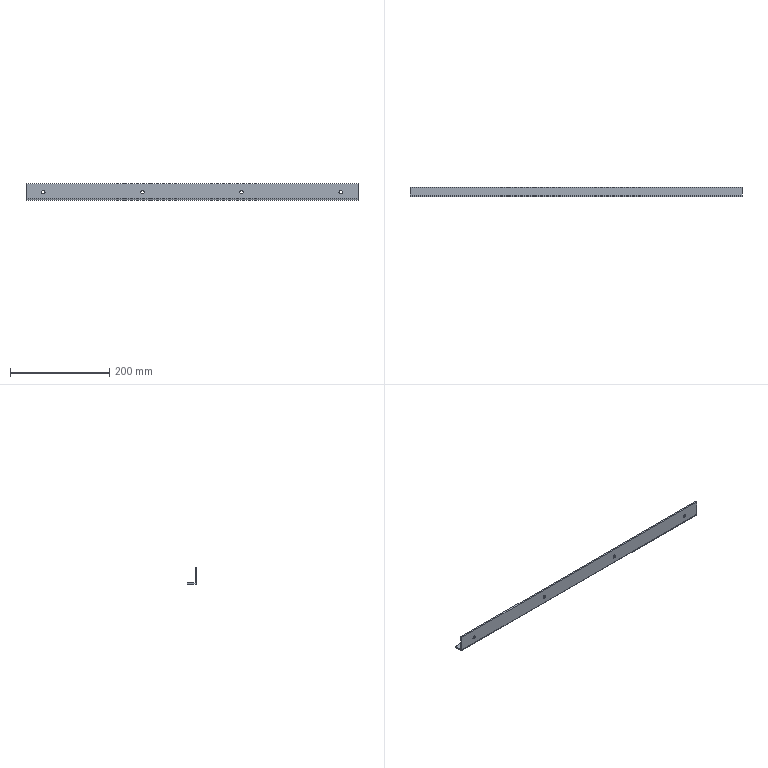Part | STEP file | HESS-408-70-15W-W-47-outer case reinforcing rib 6 | 1 solid | 18 faces | box 670 x 18.5 x 34 mm | volume 97679 mm3 | cylinder 10 | plane 8 | commonest cylinder face diameters 6.8 x8 0.2 x1 6.2 x1
STEP:
#1=CARTESIAN_POINT('',(0.,0.,0.));
#2=DIRECTION('',(0.,0.,1.));
#3=DIRECTION('',(1.,0.,0.));
#4=AXIS2_PLACEMENT_3D('',#1,#2,#3);
#5=CARTESIAN_POINT('',(-300.,0.,-3.9));
#6=VERTEX_POINT('',#5);
#7=CARTESIAN_POINT('',(-300.,-3.,-3.9));
#8=VERTEX_POINT('',#7);
#9=CARTESIAN_POINT('',(-300.,7.,-3.9));
#10=DIRECTION('',(0.,-1.,0.));
#11=VECTOR('',#10,1.);
#12=LINE('',#9,#11);
#13=CARTESIAN_POINT('',(-300.,7.,-0.5));
#14=DIRECTION('',(0.,-1.,0.));
#15=DIRECTION('',(0.,0.,-1.));
#16=AXIS2_PLACEMENT_3D('',#13,#14,#15);
#17=CYLINDRICAL_SURFACE('',#16,3.4);
#18=CARTESIAN_POINT('',(6.283,0.));
#19=DIRECTION('',(0.,1.));
#20=VECTOR('',#19,1.);
#21=LINE('',#18,#20);
#22=(GEOMETRIC_REPRESENTATION_CONTEXT(2)PARAMETRIC_REPRESENTATION_CONTEXT()REPRESENTATION_CONTEXT('',''));
#23=DEFINITIONAL_REPRESENTATION('',(#21),#22);
#24=PCURVE('',#17,#23);
#25=CARTESIAN_POINT('',(-300.,7.,-0.5));
#26=DIRECTION('',(0.,-1.,0.));
#27=DIRECTION('',(0.,0.,-1.));
#28=AXIS2_PLACEMENT_3D('',#25,#26,#27);
#29=CYLINDRICAL_SURFACE('',#28,3.4);
#30=CARTESIAN_POINT('',(0.,0.));
#31=DIRECTION('',(0.,1.));
#32=VECTOR('',#31,1.);
#33=LINE('',#30,#32);
#34=(GEOMETRIC_REPRESENTATION_CONTEXT(2)PARAMETRIC_REPRESENTATION_CONTEXT()REPRESENTATION_CONTEXT('',''));
#35=DEFINITIONAL_REPRESENTATION('',(#33),#34);
#36=PCURVE('',#29,#35);
#37=SURFACE_CURVE('',#12,(#24,#36),.PCURVE_S1.);
#38=EDGE_CURVE('',#6,#8,#37,.T.);
#39=ORIENTED_EDGE('',*,*,#38,.T.);
#40=CARTESIAN_POINT('',(-300.,-3.,2.9));
#41=VERTEX_POINT('',#40);
#42=CARTESIAN_POINT('',(-300.,-3.,-0.5));
#43=DIRECTION('',(0.,1.,0.));
#44=DIRECTION('',(0.,0.,-1.));
#45=AXIS2_PLACEMENT_3D('',#42,#43,#44);
#46=CIRCLE('',#45,3.4);
#47=CARTESIAN_POINT('',(6.283,10.));
#48=DIRECTION('',(-1.,0.));
#49=VECTOR('',#48,1.);
#50=LINE('',#47,#49);
#51=(GEOMETRIC_REPRESENTATION_CONTEXT(2)PARAMETRIC_REPRESENTATION_CONTEXT()REPRESENTATION_CONTEXT('',''));
#52=DEFINITIONAL_REPRESENTATION('',(#50),#51);
#53=PCURVE('',#17,#52);
#54=CARTESIAN_POINT('',(0.,-3.,0.));
#55=DIRECTION('',(0.,-1.,0.));
#56=DIRECTION('',(0.,0.,-1.));
#57=AXIS2_PLACEMENT_3D('',#54,#55,#56);
#58=PLANE('',#57);
#59=CARTESIAN_POINT('',(3.9,-300.));
#60=CARTESIAN_POINT('',(3.9,-305.889));
#61=CARTESIAN_POINT('',(-1.2,-302.944));
#62=CARTESIAN_POINT('',(-6.3,-300.));
#63=CARTESIAN_POINT('',(-1.2,-297.056));
#64=CARTESIAN_POINT('',(3.9,-294.111));
#65=CARTESIAN_POINT('',(3.9,-300.));
#66=(BOUNDED_CURVE()B_SPLINE_CURVE(2,(#59,#60,#61,#62,#63,#64,#65),.UNSPECIFIED.,.T.,.F.)B_SPLINE_CURVE_WITH_KNOTS((1,2,2,2,2,1),(-2.094,0.,2.094,4.189,6.283,8.378),.UNSPECIFIED.)CURVE()GEOMETRIC_REPRESENTATION_ITEM()RATIONAL_B_SPLINE_CURVE((1.,0.5,1.,0.5,1.,0.5,1.))REPRESENTATION_ITEM(''));
#67=(GEOMETRIC_REPRESENTATION_CONTEXT(2)PARAMETRIC_REPRESENTATION_CONTEXT()REPRESENTATION_CONTEXT('',''));
#68=DEFINITIONAL_REPRESENTATION('',(#66),#67);
#69=PCURVE('',#58,#68);
#70=SURFACE_CURVE('',#46,(#53,#69),.PCURVE_S1.);
#71=EDGE_CURVE('',#8,#41,#70,.T.);
#72=ORIENTED_EDGE('',*,*,#71,.T.);
#73=CARTESIAN_POINT('',(-300.,0.,2.9));
#74=VERTEX_POINT('',#73);
#75=CARTESIAN_POINT('',(-300.,7.,2.9));
#76=DIRECTION('',(0.,-1.,0.));
#77=VECTOR('',#76,1.);
#78=LINE('',#75,#77);
#79=CARTESIAN_POINT('',(3.142,0.));
#80=DIRECTION('',(0.,1.));
#81=VECTOR('',#80,1.);
#82=LINE('',#79,#81);
#83=(GEOMETRIC_REPRESENTATION_CONTEXT(2)PARAMETRIC_REPRESENTATION_CONTEXT()REPRESENTATION_CONTEXT('',''));
#84=DEFINITIONAL_REPRESENTATION('',(#82),#83);
#85=PCURVE('',#17,#84);
#86=CARTESIAN_POINT('',(3.142,0.));
#87=DIRECTION('',(0.,1.));
#88=VECTOR('',#87,1.);
#89=LINE('',#86,#88);
#90=(GEOMETRIC_REPRESENTATION_CONTEXT(2)PARAMETRIC_REPRESENTATION_CONTEXT()REPRESENTATION_CONTEXT('',''));
#91=DEFINITIONAL_REPRESENTATION('',(#89),#90);
#92=PCURVE('',#29,#91);
#93=SURFACE_CURVE('',#78,(#85,#92),.PCURVE_S1.);
#94=EDGE_CURVE('',#74,#41,#93,.T.);
#95=ORIENTED_EDGE('',*,*,#94,.F.);
#96=CARTESIAN_POINT('',(-300.,0.,-0.5));
#97=DIRECTION('',(0.,-1.,0.));
#98=DIRECTION('',(0.,0.,-1.));
#99=AXIS2_PLACEMENT_3D('',#96,#97,#98);
#100=CIRCLE('',#99,3.4);
#101=CARTESIAN_POINT('',(0.,7.));
#102=DIRECTION('',(1.,0.));
#103=VECTOR('',#102,1.);
#104=LINE('',#101,#103);
#105=(GEOMETRIC_REPRESENTATION_CONTEXT(2)PARAMETRIC_REPRESENTATION_CONTEXT()REPRESENTATION_CONTEXT('',''));
#106=DEFINITIONAL_REPRESENTATION('',(#104),#105);
#107=PCURVE('',#17,#106);
#108=CARTESIAN_POINT('',(0.,0.,0.));
#109=DIRECTION('',(0.,-1.,0.));
#110=DIRECTION('',(0.,0.,-1.));
#111=AXIS2_PLACEMENT_3D('',#108,#109,#110);
#112=PLANE('',#111);
#113=CARTESIAN_POINT('',(0.5,-300.));
#114=DIRECTION('',(1.,0.));
#115=AXIS2_PLACEMENT_2D('',#113,#114);
#116=CIRCLE('',#115,3.4);
#117=(GEOMETRIC_REPRESENTATION_CONTEXT(2)PARAMETRIC_REPRESENTATION_CONTEXT()REPRESENTATION_CONTEXT('',''));
#118=DEFINITIONAL_REPRESENTATION('',(#116),#117);
#119=PCURVE('',#112,#118);
#120=SURFACE_CURVE('',#100,(#107,#119),.PCURVE_S1.);
#121=EDGE_CURVE('',#74,#6,#120,.T.);
#122=ORIENTED_EDGE('',*,*,#121,.T.);
#123=EDGE_LOOP('',(#39,#72,#95,#122));
#124=FACE_BOUND('',#123,.F.);
#125=ADVANCED_FACE('',(#124),#17,.F.);
#126=CARTESIAN_POINT('',(300.,0.,-3.9));
#127=VERTEX_POINT('',#126);
#128=CARTESIAN_POINT('',(300.,-3.,-3.9));
#129=VERTEX_POINT('',#128);
#130=CARTESIAN_POINT('',(300.,7.,-3.9));
#131=DIRECTION('',(0.,-1.,0.));
#132=VECTOR('',#131,1.);
#133=LINE('',#130,#132);
#134=CARTESIAN_POINT('',(300.,7.,-0.5));
#135=DIRECTION('',(0.,-1.,0.));
#136=DIRECTION('',(0.,0.,-1.));
#137=AXIS2_PLACEMENT_3D('',#134,#135,#136);
#138=CYLINDRICAL_SURFACE('',#137,3.4);
#139=CARTESIAN_POINT('',(6.283,0.));
#140=DIRECTION('',(0.,1.));
#141=VECTOR('',#140,1.);
#142=LINE('',#139,#141);
#143=(GEOMETRIC_REPRESENTATION_CONTEXT(2)PARAMETRIC_REPRESENTATION_CONTEXT()REPRESENTATION_CONTEXT('',''));
#144=DEFINITIONAL_REPRESENTATION('',(#142),#143);
#145=PCURVE('',#138,#144);
#146=CARTESIAN_POINT('',(300.,7.,-0.5));
#147=DIRECTION('',(0.,-1.,0.));
#148=DIRECTION('',(0.,0.,-1.));
#149=AXIS2_PLACEMENT_3D('',#146,#147,#148);
#150=CYLINDRICAL_SURFACE('',#149,3.4);
#151=CARTESIAN_POINT('',(0.,0.));
#152=DIRECTION('',(0.,1.));
#153=VECTOR('',#152,1.);
#154=LINE('',#151,#153);
#155=(GEOMETRIC_REPRESENTATION_CONTEXT(2)PARAMETRIC_REPRESENTATION_CONTEXT()REPRESENTATION_CONTEXT('',''));
#156=DEFINITIONAL_REPRESENTATION('',(#154),#155);
#157=PCURVE('',#150,#156);
#158=SURFACE_CURVE('',#133,(#145,#157),.PCURVE_S1.);
#159=EDGE_CURVE('',#127,#129,#158,.T.);
#160=ORIENTED_EDGE('',*,*,#159,.T.);
#161=CARTESIAN_POINT('',(300.,-3.,2.9));
#162=VERTEX_POINT('',#161);
#163=CARTESIAN_POINT('',(300.,-3.,-0.5));
#164=DIRECTION('',(0.,1.,0.));
#165=DIRECTION('',(0.,0.,-1.));
#166=AXIS2_PLACEMENT_3D('',#163,#164,#165);
#167=CIRCLE('',#166,3.4);
#168=CARTESIAN_POINT('',(6.283,10.));
#169=DIRECTION('',(-1.,0.));
#170=VECTOR('',#169,1.);
#171=LINE('',#168,#170);
#172=(GEOMETRIC_REPRESENTATION_CONTEXT(2)PARAMETRIC_REPRESENTATION_CONTEXT()REPRESENTATION_CONTEXT('',''));
#173=DEFINITIONAL_REPRESENTATION('',(#171),#172);
#174=PCURVE('',#138,#173);
#175=CARTESIAN_POINT('',(3.9,300.));
#176=CARTESIAN_POINT('',(3.9,294.111));
#177=CARTESIAN_POINT('',(-1.2,297.056));
#178=CARTESIAN_POINT('',(-6.3,300.));
#179=CARTESIAN_POINT('',(-1.2,302.944));
#180=CARTESIAN_POINT('',(3.9,305.889));
#181=CARTESIAN_POINT('',(3.9,300.));
#182=(BOUNDED_CURVE()B_SPLINE_CURVE(2,(#175,#176,#177,#178,#179,#180,#181),.UNSPECIFIED.,.T.,.F.)B_SPLINE_CURVE_WITH_KNOTS((1,2,2,2,2,1),(-2.094,0.,2.094,4.189,6.283,8.378),.UNSPECIFIED.)CURVE()GEOMETRIC_REPRESENTATION_ITEM()RATIONAL_B_SPLINE_CURVE((1.,0.5,1.,0.5,1.,0.5,1.))REPRESENTATION_ITEM(''));
#183=(GEOMETRIC_REPRESENTATION_CONTEXT(2)PARAMETRIC_REPRESENTATION_CONTEXT()REPRESENTATION_CONTEXT('',''));
#184=DEFINITIONAL_REPRESENTATION('',(#182),#183);
#185=PCURVE('',#58,#184);
#186=SURFACE_CURVE('',#167,(#174,#185),.PCURVE_S1.);
#187=EDGE_CURVE('',#129,#162,#186,.T.);
#188=ORIENTED_EDGE('',*,*,#187,.T.);
#189=CARTESIAN_POINT('',(300.,0.,2.9));
#190=VERTEX_POINT('',#189);
#191=CARTESIAN_POINT('',(300.,7.,2.9));
#192=DIRECTION('',(0.,-1.,0.));
#193=VECTOR('',#192,1.);
#194=LINE('',#191,#193);
#195=CARTESIAN_POINT('',(3.142,0.));
#196=DIRECTION('',(0.,1.));
#197=VECTOR('',#196,1.);
#198=LINE('',#195,#197);
#199=(GEOMETRIC_REPRESENTATION_CONTEXT(2)PARAMETRIC_REPRESENTATION_CONTEXT()REPRESENTATION_CONTEXT('',''));
#200=DEFINITIONAL_REPRESENTATION('',(#198),#199);
#201=PCURVE('',#138,#200);
#202=CARTESIAN_POINT('',(3.142,0.));
#203=DIRECTION('',(0.,1.));
#204=VECTOR('',#203,1.);
#205=LINE('',#202,#204);
#206=(GEOMETRIC_REPRESENTATION_CONTEXT(2)PARAMETRIC_REPRESENTATION_CONTEXT()REPRESENTATION_CONTEXT('',''));
#207=DEFINITIONAL_REPRESENTATION('',(#205),#206);
#208=PCURVE('',#150,#207);
#209=SURFACE_CURVE('',#194,(#201,#208),.PCURVE_S1.);
#210=EDGE_CURVE('',#190,#162,#209,.T.);
#211=ORIENTED_EDGE('',*,*,#210,.F.);
#212=CARTESIAN_POINT('',(300.,0.,-0.5));
#213=DIRECTION('',(0.,-1.,0.));
#214=DIRECTION('',(0.,0.,-1.));
#215=AXIS2_PLACEMENT_3D('',#212,#213,#214);
#216=CIRCLE('',#215,3.4);
#217=CARTESIAN_POINT('',(0.,7.));
#218=DIRECTION('',(1.,0.));
#219=VECTOR('',#218,1.);
#220=LINE('',#217,#219);
#221=(GEOMETRIC_REPRESENTATION_CONTEXT(2)PARAMETRIC_REPRESENTATION_CONTEXT()REPRESENTATION_CONTEXT('',''));
#222=DEFINITIONAL_REPRESENTATION('',(#220),#221);
#223=PCURVE('',#138,#222);
#224=CARTESIAN_POINT('',(0.5,300.));
#225=DIRECTION('',(1.,0.));
#226=AXIS2_PLACEMENT_2D('',#224,#225);
#227=CIRCLE('',#226,3.4);
#228=(GEOMETRIC_REPRESENTATION_CONTEXT(2)PARAMETRIC_REPRESENTATION_CONTEXT()REPRESENTATION_CONTEXT('',''));
#229=DEFINITIONAL_REPRESENTATION('',(#227),#228);
#230=PCURVE('',#112,#229);
#231=SURFACE_CURVE('',#216,(#223,#230),.PCURVE_S1.);
#232=EDGE_CURVE('',#190,#127,#231,.T.);
#233=ORIENTED_EDGE('',*,*,#232,.T.);
#234=EDGE_LOOP('',(#160,#188,#211,#233));
#235=FACE_BOUND('',#234,.F.);
#236=ADVANCED_FACE('',(#235),#138,.F.);
#237=CARTESIAN_POINT('',(100.,0.,-3.9));
#238=VERTEX_POINT('',#237);
#239=CARTESIAN_POINT('',(100.,-3.,-3.9));
#240=VERTEX_POINT('',#239);
#241=CARTESIAN_POINT('',(100.,7.,-3.9));
#242=DIRECTION('',(0.,-1.,0.));
#243=VECTOR('',#242,1.);
#244=LINE('',#241,#243);
#245=CARTESIAN_POINT('',(100.,7.,-0.5));
#246=DIRECTION('',(0.,-1.,0.));
#247=DIRECTION('',(0.,0.,-1.));
#248=AXIS2_PLACEMENT_3D('',#245,#246,#247);
#249=CYLINDRICAL_SURFACE('',#248,3.4);
#250=CARTESIAN_POINT('',(6.283,0.));
#251=DIRECTION('',(0.,1.));
#252=VECTOR('',#251,1.);
#253=LINE('',#250,#252);
#254=(GEOMETRIC_REPRESENTATION_CONTEXT(2)PARAMETRIC_REPRESENTATION_CONTEXT()REPRESENTATION_CONTEXT('',''));
#255=DEFINITIONAL_REPRESENTATION('',(#253),#254);
#256=PCURVE('',#249,#255);
#257=CARTESIAN_POINT('',(100.,7.,-0.5));
#258=DIRECTION('',(0.,-1.,0.));
#259=DIRECTION('',(0.,0.,-1.));
#260=AXIS2_PLACEMENT_3D('',#257,#258,#259);
#261=CYLINDRICAL_SURFACE('',#260,3.4);
#262=CARTESIAN_POINT('',(0.,0.));
#263=DIRECTION('',(0.,1.));
#264=VECTOR('',#263,1.);
#265=LINE('',#262,#264);
#266=(GEOMETRIC_REPRESENTATION_CONTEXT(2)PARAMETRIC_REPRESENTATION_CONTEXT()REPRESENTATION_CONTEXT('',''));
#267=DEFINITIONAL_REPRESENTATION('',(#265),#266);
#268=PCURVE('',#261,#267);
#269=SURFACE_CURVE('',#244,(#256,#268),.PCURVE_S1.);
#270=EDGE_CURVE('',#238,#240,#269,.T.);
#271=ORIENTED_EDGE('',*,*,#270,.T.);
#272=CARTESIAN_POINT('',(100.,-3.,2.9));
#273=VERTEX_POINT('',#272);
#274=CARTESIAN_POINT('',(100.,-3.,-0.5));
#275=DIRECTION('',(0.,1.,0.));
#276=DIRECTION('',(0.,0.,-1.));
#277=AXIS2_PLACEMENT_3D('',#274,#275,#276);
#278=CIRCLE('',#277,3.4);
#279=CARTESIAN_POINT('',(6.283,10.));
#280=DIRECTION('',(-1.,0.));
#281=VECTOR('',#280,1.);
#282=LINE('',#279,#281);
#283=(GEOMETRIC_REPRESENTATION_CONTEXT(2)PARAMETRIC_REPRESENTATION_CONTEXT()REPRESENTATION_CONTEXT('',''));
#284=DEFINITIONAL_REPRESENTATION('',(#282),#283);
#285=PCURVE('',#249,#284);
#286=CARTESIAN_POINT('',(3.9,100.));
#287=CARTESIAN_POINT('',(3.9,94.111));
#288=CARTESIAN_POINT('',(-1.2,97.056));
#289=CARTESIAN_POINT('',(-6.3,100.));
#290=CARTESIAN_POINT('',(-1.2,102.944));
#291=CARTESIAN_POINT('',(3.9,105.889));
#292=CARTESIAN_POINT('',(3.9,100.));
#293=(BOUNDED_CURVE()B_SPLINE_CURVE(2,(#286,#287,#288,#289,#290,#291,#292),.UNSPECIFIED.,.T.,.F.)B_SPLINE_CURVE_WITH_KNOTS((1,2,2,2,2,1),(-2.094,0.,2.094,4.189,6.283,8.378),.UNSPECIFIED.)CURVE()GEOMETRIC_REPRESENTATION_ITEM()RATIONAL_B_SPLINE_CURVE((1.,0.5,1.,0.5,1.,0.5,1.))REPRESENTATION_ITEM(''));
#294=(GEOMETRIC_REPRESENTATION_CONTEXT(2)PARAMETRIC_REPRESENTATION_CONTEXT()REPRESENTATION_CONTEXT('',''));
#295=DEFINITIONAL_REPRESENTATION('',(#293),#294);
#296=PCURVE('',#58,#295);
#297=SURFACE_CURVE('',#278,(#285,#296),.PCURVE_S1.);
#298=EDGE_CURVE('',#240,#273,#297,.T.);
#299=ORIENTED_EDGE('',*,*,#298,.T.);
#300=CARTESIAN_POINT('',(100.,0.,2.9));
#301=VERTEX_POINT('',#300);
#302=CARTESIAN_POINT('',(100.,7.,2.9));
#303=DIRECTION('',(0.,-1.,0.));
#304=VECTOR('',#303,1.);
#305=LINE('',#302,#304);
#306=CARTESIAN_POINT('',(3.142,0.));
#307=DIRECTION('',(0.,1.));
#308=VECTOR('',#307,1.);
#309=LINE('',#306,#308);
#310=(GEOMETRIC_REPRESENTATION_CONTEXT(2)PARAMETRIC_REPRESENTATION_CONTEXT()REPRESENTATION_CONTEXT('',''));
#311=DEFINITIONAL_REPRESENTATION('',(#309),#310);
#312=PCURVE('',#249,#311);
#313=CARTESIAN_POINT('',(3.142,0.));
#314=DIRECTION('',(0.,1.));
#315=VECTOR('',#314,1.);
#316=LINE('',#313,#315);
#317=(GEOMETRIC_REPRESENTATION_CONTEXT(2)PARAMETRIC_REPRESENTATION_CONTEXT()REPRESENTATION_CONTEXT('',''));
#318=DEFINITIONAL_REPRESENTATION('',(#316),#317);
#319=PCURVE('',#261,#318);
#320=SURFACE_CURVE('',#305,(#312,#319),.PCURVE_S1.);
#321=EDGE_CURVE('',#301,#273,#320,.T.);
#322=ORIENTED_EDGE('',*,*,#321,.F.);
#323=CARTESIAN_POINT('',(100.,0.,-0.5));
#324=DIRECTION('',(0.,-1.,0.));
#325=DIRECTION('',(0.,0.,-1.));
#326=AXIS2_PLACEMENT_3D('',#323,#324,#325);
#327=CIRCLE('',#326,3.4);
#328=CARTESIAN_POINT('',(0.,7.));
#329=DIRECTION('',(1.,0.));
#330=VECTOR('',#329,1.);
#331=LINE('',#328,#330);
#332=(GEOMETRIC_REPRESENTATION_CONTEXT(2)PARAMETRIC_REPRESENTATION_CONTEXT()REPRESENTATION_CONTEXT('',''));
#333=DEFINITIONAL_REPRESENTATION('',(#331),#332);
#334=PCURVE('',#249,#333);
#335=CARTESIAN_POINT('',(0.5,100.));
#336=DIRECTION('',(1.,0.));
#337=AXIS2_PLACEMENT_2D('',#335,#336);
#338=CIRCLE('',#337,3.4);
#339=(GEOMETRIC_REPRESENTATION_CONTEXT(2)PARAMETRIC_REPRESENTATION_CONTEXT()REPRESENTATION_CONTEXT('',''));
#340=DEFINITIONAL_REPRESENTATION('',(#338),#339);
#341=PCURVE('',#112,#340);
#342=SURFACE_CURVE('',#327,(#334,#341),.PCURVE_S1.);
#343=EDGE_CURVE('',#301,#238,#342,.T.);
#344=ORIENTED_EDGE('',*,*,#343,.T.);
#345=EDGE_LOOP('',(#271,#299,#322,#344));
#346=FACE_BOUND('',#345,.F.);
#347=ADVANCED_FACE('',(#346),#249,.F.);
#348=CARTESIAN_POINT('',(-100.,0.,-3.9));
#349=VERTEX_POINT('',#348);
#350=CARTESIAN_POINT('',(-100.,-3.,-3.9));
#351=VERTEX_POINT('',#350);
#352=CARTESIAN_POINT('',(-100.,7.,-3.9));
#353=DIRECTION('',(0.,-1.,0.));
#354=VECTOR('',#353,1.);
#355=LINE('',#352,#354);
#356=CARTESIAN_POINT('',(-100.,7.,-0.5));
#357=DIRECTION('',(0.,-1.,0.));
#358=DIRECTION('',(0.,0.,-1.));
#359=AXIS2_PLACEMENT_3D('',#356,#357,#358);
#360=CYLINDRICAL_SURFACE('',#359,3.4);
#361=CARTESIAN_POINT('',(6.283,0.));
#362=DIRECTION('',(0.,1.));
#363=VECTOR('',#362,1.);
#364=LINE('',#361,#363);
#365=(GEOMETRIC_REPRESENTATION_CONTEXT(2)PARAMETRIC_REPRESENTATION_CONTEXT()REPRESENTATION_CONTEXT('',''));
#366=DEFINITIONAL_REPRESENTATION('',(#364),#365);
#367=PCURVE('',#360,#366);
#368=CARTESIAN_POINT('',(-100.,7.,-0.5));
#369=DIRECTION('',(0.,-1.,0.));
#370=DIRECTION('',(0.,0.,-1.));
#371=AXIS2_PLACEMENT_3D('',#368,#369,#370);
#372=CYLINDRICAL_SURFACE('',#371,3.4);
#373=CARTESIAN_POINT('',(0.,0.));
#374=DIRECTION('',(0.,1.));
#375=VECTOR('',#374,1.);
#376=LINE('',#373,#375);
#377=(GEOMETRIC_REPRESENTATION_CONTEXT(2)PARAMETRIC_REPRESENTATION_CONTEXT()REPRESENTATION_CONTEXT('',''));
#378=DEFINITIONAL_REPRESENTATION('',(#376),#377);
#379=PCURVE('',#372,#378);
#380=SURFACE_CURVE('',#355,(#367,#379),.PCURVE_S1.);
#381=EDGE_CURVE('',#349,#351,#380,.T.);
#382=ORIENTED_EDGE('',*,*,#381,.T.);
#383=CARTESIAN_POINT('',(-100.,-3.,2.9));
#384=VERTEX_POINT('',#383);
#385=CARTESIAN_POINT('',(-100.,-3.,-0.5));
#386=DIRECTION('',(0.,1.,0.));
#387=DIRECTION('',(0.,0.,-1.));
#388=AXIS2_PLACEMENT_3D('',#385,#386,#387);
#389=CIRCLE('',#388,3.4);
#390=CARTESIAN_POINT('',(6.283,10.));
#391=DIRECTION('',(-1.,0.));
#392=VECTOR('',#391,1.);
#393=LINE('',#390,#392);
#394=(GEOMETRIC_REPRESENTATION_CONTEXT(2)PARAMETRIC_REPRESENTATION_CONTEXT()REPRESENTATION_CONTEXT('',''));
#395=DEFINITIONAL_REPRESENTATION('',(#393),#394);
#396=PCURVE('',#360,#395);
#397=CARTESIAN_POINT('',(3.9,-100.));
#398=CARTESIAN_POINT('',(3.9,-105.889));
#399=CARTESIAN_POINT('',(-1.2,-102.944));
#400=CARTESIAN_POINT('',(-6.3,-100.));
#401=CARTESIAN_POINT('',(-1.2,-97.056));
#402=CARTESIAN_POINT('',(3.9,-94.111));
#403=CARTESIAN_POINT('',(3.9,-100.));
#404=(BOUNDED_CURVE()B_SPLINE_CURVE(2,(#397,#398,#399,#400,#401,#402,#403),.UNSPECIFIED.,.T.,.F.)B_SPLINE_CURVE_WITH_KNOTS((1,2,2,2,2,1),(-2.094,0.,2.094,4.189,6.283,8.378),.UNSPECIFIED.)CURVE()GEOMETRIC_REPRESENTATION_ITEM()RATIONAL_B_SPLINE_CURVE((1.,0.5,1.,0.5,1.,0.5,1.))REPRESENTATION_ITEM(''));
#405=(GEOMETRIC_REPRESENTATION_CONTEXT(2)PARAMETRIC_REPRESENTATION_CONTEXT()REPRESENTATION_CONTEXT('',''));
#406=DEFINITIONAL_REPRESENTATION('',(#404),#405);
#407=PCURVE('',#58,#406);
#408=SURFACE_CURVE('',#389,(#396,#407),.PCURVE_S1.);
#409=EDGE_CURVE('',#351,#384,#408,.T.);
#410=ORIENTED_EDGE('',*,*,#409,.T.);
#411=CARTESIAN_POINT('',(-100.,0.,2.9));
#412=VERTEX_POINT('',#411);
#413=CARTESIAN_POINT('',(-100.,7.,2.9));
#414=DIRECTION('',(0.,-1.,0.));
#415=VECTOR('',#414,1.);
#416=LINE('',#413,#415);
#417=CARTESIAN_POINT('',(3.142,0.));
#418=DIRECTION('',(0.,1.));
#419=VECTOR('',#418,1.);
#420=LINE('',#417,#419);
#421=(GEOMETRIC_REPRESENTATION_CONTEXT(2)PARAMETRIC_REPRESENTATION_CONTEXT()REPRESENTATION_CONTEXT('',''));
#422=DEFINITIONAL_REPRESENTATION('',(#420),#421);
#423=PCURVE('',#360,#422);
#424=CARTESIAN_POINT('',(3.142,0.));
#425=DIRECTION('',(0.,1.));
#426=VECTOR('',#425,1.);
#427=LINE('',#424,#426);
#428=(GEOMETRIC_REPRESENTATION_CONTEXT(2)PARAMETRIC_REPRESENTATION_CONTEXT()REPRESENTATION_CONTEXT('',''));
#429=DEFINITIONAL_REPRESENTATION('',(#427),#428);
#430=PCURVE('',#372,#429);
#431=SURFACE_CURVE('',#416,(#423,#430),.PCURVE_S1.);
#432=EDGE_CURVE('',#412,#384,#431,.T.);
#433=ORIENTED_EDGE('',*,*,#432,.F.);
#434=CARTESIAN_POINT('',(-100.,0.,-0.5));
#435=DIRECTION('',(0.,-1.,0.));
#436=DIRECTION('',(0.,0.,-1.));
#437=AXIS2_PLACEMENT_3D('',#434,#435,#436);
#438=CIRCLE('',#437,3.4);
#439=CARTESIAN_POINT('',(0.,7.));
#440=DIRECTION('',(1.,0.));
#441=VECTOR('',#440,1.);
#442=LINE('',#439,#441);
#443=(GEOMETRIC_REPRESENTATION_CONTEXT(2)PARAMETRIC_REPRESENTATION_CONTEXT()REPRESENTATION_CONTEXT('',''));
#444=DEFINITIONAL_REPRESENTATION('',(#442),#443);
#445=PCURVE('',#360,#444);
#446=CARTESIAN_POINT('',(0.5,-100.));
#447=DIRECTION('',(1.,0.));
#448=AXIS2_PLACEMENT_2D('',#446,#447);
#449=CIRCLE('',#448,3.4);
#450=(GEOMETRIC_REPRESENTATION_CONTEXT(2)PARAMETRIC_REPRESENTATION_CONTEXT()REPRESENTATION_CONTEXT('',''));
#451=DEFINITIONAL_REPRESENTATION('',(#449),#450);
#452=PCURVE('',#112,#451);
#453=SURFACE_CURVE('',#438,(#445,#452),.PCURVE_S1.);
#454=EDGE_CURVE('',#412,#349,#453,.T.);
#455=ORIENTED_EDGE('',*,*,#454,.T.);
#456=EDGE_LOOP('',(#382,#410,#433,#455));
#457=FACE_BOUND('',#456,.F.);
#458=ADVANCED_FACE('',(#457),#360,.F.);
#459=CARTESIAN_POINT('',(335.,-3.,-13.9));
#460=VERTEX_POINT('',#459);
#461=CARTESIAN_POINT('',(335.,-3.,17.));
#462=VERTEX_POINT('',#461);
#463=CARTESIAN_POINT('',(335.,-3.,0.));
#464=DIRECTION('',(0.,0.,1.));
#465=VECTOR('',#464,1.);
#466=LINE('',#463,#465);
#467=CARTESIAN_POINT('',(0.,335.));
#468=DIRECTION('',(-1.,0.));
#469=VECTOR('',#468,1.);
#470=LINE('',#467,#469);
#471=(GEOMETRIC_REPRESENTATION_CONTEXT(2)PARAMETRIC_REPRESENTATION_CONTEXT()REPRESENTATION_CONTEXT('',''));
#472=DEFINITIONAL_REPRESENTATION('',(#470),#471);
#473=PCURVE('',#58,#472);
#474=CARTESIAN_POINT('',(335.,-3.,17.));
#475=DIRECTION('',(1.,0.,0.));
#476=DIRECTION('',(0.,0.,-1.));
#477=AXIS2_PLACEMENT_3D('',#474,#475,#476);
#478=PLANE('',#477);
#479=CARTESIAN_POINT('',(17.,0.));
#480=DIRECTION('',(-1.,0.));
#481=VECTOR('',#480,1.);
#482=LINE('',#479,#481);
#483=(GEOMETRIC_REPRESENTATION_CONTEXT(2)PARAMETRIC_REPRESENTATION_CONTEXT()REPRESENTATION_CONTEXT('',''));
#484=DEFINITIONAL_REPRESENTATION('',(#482),#483);
#485=PCURVE('',#478,#484);
#486=SURFACE_CURVE('',#466,(#473,#485),.PCURVE_S1.);
#487=EDGE_CURVE('',#460,#462,#486,.T.);
#488=ORIENTED_EDGE('',*,*,#487,.T.);
#489=CARTESIAN_POINT('',(-335.,-3.,17.));
#490=VERTEX_POINT('',#489);
#491=CARTESIAN_POINT('',(0.,-3.,17.));
#492=DIRECTION('',(-1.,0.,0.));
#493=VECTOR('',#492,1.);
#494=LINE('',#491,#493);
#495=CARTESIAN_POINT('',(-17.,0.));
#496=DIRECTION('',(0.,-1.));
#497=VECTOR('',#496,1.);
#498=LINE('',#495,#497);
#499=(GEOMETRIC_REPRESENTATION_CONTEXT(2)PARAMETRIC_REPRESENTATION_CONTEXT()REPRESENTATION_CONTEXT('',''));
#500=DEFINITIONAL_REPRESENTATION('',(#498),#499);
#501=PCURVE('',#58,#500);
#502=CARTESIAN_POINT('',(-335.,-3.,17.));
#503=DIRECTION('',(0.,0.,1.));
#504=DIRECTION('',(1.,0.,0.));
#505=AXIS2_PLACEMENT_3D('',#502,#503,#504);
#506=PLANE('',#505);
#507=CARTESIAN_POINT('',(335.,0.));
#508=DIRECTION('',(-1.,0.));
#509=VECTOR('',#508,1.);
#510=LINE('',#507,#509);
#511=(GEOMETRIC_REPRESENTATION_CONTEXT(2)PARAMETRIC_REPRESENTATION_CONTEXT()REPRESENTATION_CONTEXT('',''));
#512=DEFINITIONAL_REPRESENTATION('',(#510),#511);
#513=PCURVE('',#506,#512);
#514=SURFACE_CURVE('',#494,(#501,#513),.PCURVE_S1.);
#515=EDGE_CURVE('',#462,#490,#514,.T.);
#516=ORIENTED_EDGE('',*,*,#515,.T.);
#517=CARTESIAN_POINT('',(-335.,-3.,-13.9));
#518=VERTEX_POINT('',#517);
#519=CARTESIAN_POINT('',(-335.,-3.,0.));
#520=DIRECTION('',(0.,0.,-1.));
#521=VECTOR('',#520,1.);
#522=LINE('',#519,#521);
#523=CARTESIAN_POINT('',(0.,-335.));
#524=DIRECTION('',(1.,0.));
#525=VECTOR('',#524,1.);
#526=LINE('',#523,#525);
#527=(GEOMETRIC_REPRESENTATION_CONTEXT(2)PARAMETRIC_REPRESENTATION_CONTEXT()REPRESENTATION_CONTEXT('',''));
#528=DEFINITIONAL_REPRESENTATION('',(#526),#527);
#529=PCURVE('',#58,#528);
#530=CARTESIAN_POINT('',(-335.,-3.,17.));
#531=DIRECTION('',(-1.,0.,0.));
#532=DIRECTION('',(0.,0.,1.));
#533=AXIS2_PLACEMENT_3D('',#530,#531,#532);
#534=PLANE('',#533);
#535=CARTESIAN_POINT('',(-17.,0.));
#536=DIRECTION('',(-1.,0.));
#537=VECTOR('',#536,1.);
#538=LINE('',#535,#537);
#539=(GEOMETRIC_REPRESENTATION_CONTEXT(2)PARAMETRIC_REPRESENTATION_CONTEXT()REPRESENTATION_CONTEXT('',''));
#540=DEFINITIONAL_REPRESENTATION('',(#538),#539);
#541=PCURVE('',#534,#540);
#542=SURFACE_CURVE('',#522,(#529,#541),.PCURVE_S1.);
#543=EDGE_CURVE('',#490,#518,#542,.T.);
#544=ORIENTED_EDGE('',*,*,#543,.T.);
#545=CARTESIAN_POINT('',(0.,-3.,-13.9));
#546=DIRECTION('',(1.,0.,0.));
#547=VECTOR('',#546,1.);
#548=LINE('',#545,#547);
#549=CARTESIAN_POINT('',(13.9,0.));
#550=DIRECTION('',(0.,1.));
#551=VECTOR('',#550,1.);
#552=LINE('',#549,#551);
#553=(GEOMETRIC_REPRESENTATION_CONTEXT(2)PARAMETRIC_REPRESENTATION_CONTEXT()REPRESENTATION_CONTEXT('',''));
#554=DEFINITIONAL_REPRESENTATION('',(#552),#553);
#555=PCURVE('',#58,#554);
#556=CARTESIAN_POINT('',(-335.,0.1,-13.9));
#557=DIRECTION('',(-1.,0.,0.));
#558=DIRECTION('',(0.,0.,1.));
#559=AXIS2_PLACEMENT_3D('',#556,#557,#558);
#560=CYLINDRICAL_SURFACE('',#559,3.1);
#561=CARTESIAN_POINT('',(4.712,-335.));
#562=DIRECTION('',(0.,-1.));
#563=VECTOR('',#562,1.);
#564=LINE('',#561,#563);
#565=(GEOMETRIC_REPRESENTATION_CONTEXT(2)PARAMETRIC_REPRESENTATION_CONTEXT()REPRESENTATION_CONTEXT('',''));
#566=DEFINITIONAL_REPRESENTATION('',(#564),#565);
#567=PCURVE('',#560,#566);
#568=SURFACE_CURVE('',#548,(#555,#567),.PCURVE_S1.);
#569=EDGE_CURVE('',#518,#460,#568,.T.);
#570=ORIENTED_EDGE('',*,*,#569,.T.);
#571=EDGE_LOOP('',(#488,#516,#544,#570));
#572=FACE_BOUND('',#571,.T.);
#573=ORIENTED_EDGE('',*,*,#71,.T.);
#574=CARTESIAN_POINT('',(-300.,-3.,-0.5));
#575=DIRECTION('',(0.,1.,0.));
#576=DIRECTION('',(0.,0.,-1.));
#577=AXIS2_PLACEMENT_3D('',#574,#575,#576);
#578=CIRCLE('',#577,3.4);
#579=CARTESIAN_POINT('',(3.9,-300.));
#580=CARTESIAN_POINT('',(3.9,-305.889));
#581=CARTESIAN_POINT('',(-1.2,-302.944));
#582=CARTESIAN_POINT('',(-6.3,-300.));
#583=CARTESIAN_POINT('',(-1.2,-297.056));
#584=CARTESIAN_POINT('',(3.9,-294.111));
#585=CARTESIAN_POINT('',(3.9,-300.));
#586=(BOUNDED_CURVE()B_SPLINE_CURVE(2,(#579,#580,#581,#582,#583,#584,#585),.UNSPECIFIED.,.T.,.F.)B_SPLINE_CURVE_WITH_KNOTS((1,2,2,2,2,1),(-2.094,0.,2.094,4.189,6.283,8.378),.UNSPECIFIED.)CURVE()GEOMETRIC_REPRESENTATION_ITEM()RATIONAL_B_SPLINE_CURVE((1.,0.5,1.,0.5,1.,0.5,1.))REPRESENTATION_ITEM(''));
#587=(GEOMETRIC_REPRESENTATION_CONTEXT(2)PARAMETRIC_REPRESENTATION_CONTEXT()REPRESENTATION_CONTEXT('',''));
#588=DEFINITIONAL_REPRESENTATION('',(#586),#587);
#589=PCURVE('',#58,#588);
#590=CARTESIAN_POINT('',(6.283,10.));
#591=DIRECTION('',(-1.,0.));
#592=VECTOR('',#591,1.);
#593=LINE('',#590,#592);
#594=(GEOMETRIC_REPRESENTATION_CONTEXT(2)PARAMETRIC_REPRESENTATION_CONTEXT()REPRESENTATION_CONTEXT('',''));
#595=DEFINITIONAL_REPRESENTATION('',(#593),#594);
#596=PCURVE('',#29,#595);
#597=SURFACE_CURVE('',#578,(#589,#596),.PCURVE_S1.);
#598=EDGE_CURVE('',#41,#8,#597,.T.);
#599=ORIENTED_EDGE('',*,*,#598,.T.);
#600=EDGE_LOOP('',(#573,#599));
#601=FACE_BOUND('',#600,.T.);
#602=ORIENTED_EDGE('',*,*,#187,.T.);
#603=CARTESIAN_POINT('',(300.,-3.,-0.5));
#604=DIRECTION('',(0.,1.,0.));
#605=DIRECTION('',(0.,0.,-1.));
#606=AXIS2_PLACEMENT_3D('',#603,#604,#605);
#607=CIRCLE('',#606,3.4);
#608=CARTESIAN_POINT('',(3.9,300.));
#609=CARTESIAN_POINT('',(3.9,294.111));
#610=CARTESIAN_POINT('',(-1.2,297.056));
#611=CARTESIAN_POINT('',(-6.3,300.));
#612=CARTESIAN_POINT('',(-1.2,302.944));
#613=CARTESIAN_POINT('',(3.9,305.889));
#614=CARTESIAN_POINT('',(3.9,300.));
#615=(BOUNDED_CURVE()B_SPLINE_CURVE(2,(#608,#609,#610,#611,#612,#613,#614),.UNSPECIFIED.,.T.,.F.)B_SPLINE_CURVE_WITH_KNOTS((1,2,2,2,2,1),(-2.094,0.,2.094,4.189,6.283,8.378),.UNSPECIFIED.)CURVE()GEOMETRIC_REPRESENTATION_ITEM()RATIONAL_B_SPLINE_CURVE((1.,0.5,1.,0.5,1.,0.5,1.))REPRESENTATION_ITEM(''));
#616=(GEOMETRIC_REPRESENTATION_CONTEXT(2)PARAMETRIC_REPRESENTATION_CONTEXT()REPRESENTATION_CONTEXT('',''));
#617=DEFINITIONAL_REPRESENTATION('',(#615),#616);
#618=PCURVE('',#58,#617);
#619=CARTESIAN_POINT('',(6.283,10.));
#620=DIRECTION('',(-1.,0.));
#621=VECTOR('',#620,1.);
#622=LINE('',#619,#621);
#623=(GEOMETRIC_REPRESENTATION_CONTEXT(2)PARAMETRIC_REPRESENTATION_CONTEXT()REPRESENTATION_CONTEXT('',''));
#624=DEFINITIONAL_REPRESENTATION('',(#622),#623);
#625=PCURVE('',#150,#624);
#626=SURFACE_CURVE('',#607,(#618,#625),.PCURVE_S1.);
#627=EDGE_CURVE('',#162,#129,#626,.T.);
#628=ORIENTED_EDGE('',*,*,#627,.T.);
#629=EDGE_LOOP('',(#602,#628));
#630=FACE_BOUND('',#629,.T.);
#631=ORIENTED_EDGE('',*,*,#298,.T.);
#632=CARTESIAN_POINT('',(100.,-3.,-0.5));
#633=DIRECTION('',(0.,1.,0.));
#634=DIRECTION('',(0.,0.,-1.));
#635=AXIS2_PLACEMENT_3D('',#632,#633,#634);
#636=CIRCLE('',#635,3.4);
#637=CARTESIAN_POINT('',(3.9,100.));
#638=CARTESIAN_POINT('',(3.9,94.111));
#639=CARTESIAN_POINT('',(-1.2,97.056));
#640=CARTESIAN_POINT('',(-6.3,100.));
#641=CARTESIAN_POINT('',(-1.2,102.944));
#642=CARTESIAN_POINT('',(3.9,105.889));
#643=CARTESIAN_POINT('',(3.9,100.));
#644=(BOUNDED_CURVE()B_SPLINE_CURVE(2,(#637,#638,#639,#640,#641,#642,#643),.UNSPECIFIED.,.T.,.F.)B_SPLINE_CURVE_WITH_KNOTS((1,2,2,2,2,1),(-2.094,0.,2.094,4.189,6.283,8.378),.UNSPECIFIED.)CURVE()GEOMETRIC_REPRESENTATION_ITEM()RATIONAL_B_SPLINE_CURVE((1.,0.5,1.,0.5,1.,0.5,1.))REPRESENTATION_ITEM(''));
#645=(GEOMETRIC_REPRESENTATION_CONTEXT(2)PARAMETRIC_REPRESENTATION_CONTEXT()REPRESENTATION_CONTEXT('',''));
#646=DEFINITIONAL_REPRESENTATION('',(#644),#645);
#647=PCURVE('',#58,#646);
#648=CARTESIAN_POINT('',(6.283,10.));
#649=DIRECTION('',(-1.,0.));
#650=VECTOR('',#649,1.);
#651=LINE('',#648,#650);
#652=(GEOMETRIC_REPRESENTATION_CONTEXT(2)PARAMETRIC_REPRESENTATION_CONTEXT()REPRESENTATION_CONTEXT('',''));
#653=DEFINITIONAL_REPRESENTATION('',(#651),#652);
#654=PCURVE('',#261,#653);
#655=SURFACE_CURVE('',#636,(#647,#654),.PCURVE_S1.);
#656=EDGE_CURVE('',#273,#240,#655,.T.);
#657=ORIENTED_EDGE('',*,*,#656,.T.);
#658=EDGE_LOOP('',(#631,#657));
#659=FACE_BOUND('',#658,.T.);
#660=ORIENTED_EDGE('',*,*,#409,.T.);
#661=CARTESIAN_POINT('',(-100.,-3.,-0.5));
#662=DIRECTION('',(0.,1.,0.));
#663=DIRECTION('',(0.,0.,-1.));
#664=AXIS2_PLACEMENT_3D('',#661,#662,#663);
#665=CIRCLE('',#664,3.4);
#666=CARTESIAN_POINT('',(3.9,-100.));
#667=CARTESIAN_POINT('',(3.9,-105.889));
#668=CARTESIAN_POINT('',(-1.2,-102.944));
#669=CARTESIAN_POINT('',(-6.3,-100.));
#670=CARTESIAN_POINT('',(-1.2,-97.056));
#671=CARTESIAN_POINT('',(3.9,-94.111));
#672=CARTESIAN_POINT('',(3.9,-100.));
#673=(BOUNDED_CURVE()B_SPLINE_CURVE(2,(#666,#667,#668,#669,#670,#671,#672),.UNSPECIFIED.,.T.,.F.)B_SPLINE_CURVE_WITH_KNOTS((1,2,2,2,2,1),(-2.094,0.,2.094,4.189,6.283,8.378),.UNSPECIFIED.)CURVE()GEOMETRIC_REPRESENTATION_ITEM()RATIONAL_B_SPLINE_CURVE((1.,0.5,1.,0.5,1.,0.5,1.))REPRESENTATION_ITEM(''));
#674=(GEOMETRIC_REPRESENTATION_CONTEXT(2)PARAMETRIC_REPRESENTATION_CONTEXT()REPRESENTATION_CONTEXT('',''));
#675=DEFINITIONAL_REPRESENTATION('',(#673),#674);
#676=PCURVE('',#58,#675);
#677=CARTESIAN_POINT('',(6.283,10.));
#678=DIRECTION('',(-1.,0.));
#679=VECTOR('',#678,1.);
#680=LINE('',#677,#679);
#681=(GEOMETRIC_REPRESENTATION_CONTEXT(2)PARAMETRIC_REPRESENTATION_CONTEXT()REPRESENTATION_CONTEXT('',''));
#682=DEFINITIONAL_REPRESENTATION('',(#680),#681);
#683=PCURVE('',#372,#682);
#684=SURFACE_CURVE('',#665,(#676,#683),.PCURVE_S1.);
#685=EDGE_CURVE('',#384,#351,#684,.T.);
#686=ORIENTED_EDGE('',*,*,#685,.T.);
#687=EDGE_LOOP('',(#660,#686));
#688=FACE_BOUND('',#687,.T.);
#689=ADVANCED_FACE('',(#572,#601,#630,#659,#688),#58,.T.);
#690=ORIENTED_EDGE('',*,*,#515,.F.);
#691=CARTESIAN_POINT('',(335.,0.,17.));
#692=VERTEX_POINT('',#691);
#693=CARTESIAN_POINT('',(335.,-3.,17.));
#694=DIRECTION('',(0.,1.,0.));
#695=VECTOR('',#694,1.);
#696=LINE('',#693,#695);
#697=CARTESIAN_POINT('',(670.,0.));
#698=DIRECTION('',(0.,1.));
#699=VECTOR('',#698,1.);
#700=LINE('',#697,#699);
#701=(GEOMETRIC_REPRESENTATION_CONTEXT(2)PARAMETRIC_REPRESENTATION_CONTEXT()REPRESENTATION_CONTEXT('',''));
#702=DEFINITIONAL_REPRESENTATION('',(#700),#701);
#703=PCURVE('',#506,#702);
#704=CARTESIAN_POINT('',(0.,0.));
#705=DIRECTION('',(0.,1.));
#706=VECTOR('',#705,1.);
#707=LINE('',#704,#706);
#708=(GEOMETRIC_REPRESENTATION_CONTEXT(2)PARAMETRIC_REPRESENTATION_CONTEXT()REPRESENTATION_CONTEXT('',''));
#709=DEFINITIONAL_REPRESENTATION('',(#707),#708);
#710=PCURVE('',#478,#709);
#711=SURFACE_CURVE('',#696,(#703,#710),.PCURVE_S1.);
#712=EDGE_CURVE('',#462,#692,#711,.T.);
#713=ORIENTED_EDGE('',*,*,#712,.T.);
#714=CARTESIAN_POINT('',(-335.,0.,17.));
#715=VERTEX_POINT('',#714);
#716=CARTESIAN_POINT('',(-335.,0.,17.));
#717=DIRECTION('',(-1.,0.,0.));
#718=VECTOR('',#717,1.);
#719=LINE('',#716,#718);
#720=CARTESIAN_POINT('',(0.,3.));
#721=DIRECTION('',(-1.,0.));
#722=VECTOR('',#721,1.);
#723=LINE('',#720,#722);
#724=(GEOMETRIC_REPRESENTATION_CONTEXT(2)PARAMETRIC_REPRESENTATION_CONTEXT()REPRESENTATION_CONTEXT('',''));
#725=DEFINITIONAL_REPRESENTATION('',(#723),#724);
#726=PCURVE('',#506,#725);
#727=CARTESIAN_POINT('',(-17.,-335.));
#728=DIRECTION('',(0.,-1.));
#729=VECTOR('',#728,1.);
#730=LINE('',#727,#729);
#731=(GEOMETRIC_REPRESENTATION_CONTEXT(2)PARAMETRIC_REPRESENTATION_CONTEXT()REPRESENTATION_CONTEXT('',''));
#732=DEFINITIONAL_REPRESENTATION('',(#730),#731);
#733=PCURVE('',#112,#732);
#734=SURFACE_CURVE('',#719,(#726,#733),.PCURVE_S1.);
#735=EDGE_CURVE('',#692,#715,#734,.T.);
#736=ORIENTED_EDGE('',*,*,#735,.T.);
#737=CARTESIAN_POINT('',(-335.,-3.,17.));
#738=DIRECTION('',(0.,-1.,0.));
#739=VECTOR('',#738,1.);
#740=LINE('',#737,#739);
#741=CARTESIAN_POINT('',(0.,0.));
#742=DIRECTION('',(0.,-1.));
#743=VECTOR('',#742,1.);
#744=LINE('',#741,#743);
#745=(GEOMETRIC_REPRESENTATION_CONTEXT(2)PARAMETRIC_REPRESENTATION_CONTEXT()REPRESENTATION_CONTEXT('',''));
#746=DEFINITIONAL_REPRESENTATION('',(#744),#745);
#747=PCURVE('',#506,#746);
#748=CARTESIAN_POINT('',(0.,0.));
#749=DIRECTION('',(0.,-1.));
#750=VECTOR('',#749,1.);
#751=LINE('',#748,#750);
#752=(GEOMETRIC_REPRESENTATION_CONTEXT(2)PARAMETRIC_REPRESENTATION_CONTEXT()REPRESENTATION_CONTEXT('',''));
#753=DEFINITIONAL_REPRESENTATION('',(#751),#752);
#754=PCURVE('',#534,#753);
#755=SURFACE_CURVE('',#740,(#747,#754),.PCURVE_S1.);
#756=EDGE_CURVE('',#715,#490,#755,.T.);
#757=ORIENTED_EDGE('',*,*,#756,.T.);
#758=EDGE_LOOP('',(#690,#713,#736,#757));
#759=FACE_BOUND('',#758,.T.);
#760=ADVANCED_FACE('',(#759),#506,.T.);
#761=ORIENTED_EDGE('',*,*,#712,.F.);
#762=ORIENTED_EDGE('',*,*,#487,.F.);
#763=CARTESIAN_POINT('',(335.,0.1,-17.));
#764=VERTEX_POINT('',#763);
#765=CARTESIAN_POINT('',(335.,0.1,-13.9));
#766=DIRECTION('',(-1.,0.,0.));
#767=DIRECTION('',(0.,0.,1.));
#768=AXIS2_PLACEMENT_3D('',#765,#766,#767);
#769=CIRCLE('',#768,3.1);
#770=CARTESIAN_POINT('',(27.8,3.1));
#771=CARTESIAN_POINT('',(27.8,8.469));
#772=CARTESIAN_POINT('',(32.45,5.785));
#773=CARTESIAN_POINT('',(37.1,3.1));
#774=CARTESIAN_POINT('',(32.45,0.4153));
#775=CARTESIAN_POINT('',(27.8,-2.269));
#776=CARTESIAN_POINT('',(27.8,3.1));
#777=(BOUNDED_CURVE()B_SPLINE_CURVE(2,(#770,#771,#772,#773,#774,#775,#776),.UNSPECIFIED.,.T.,.F.)B_SPLINE_CURVE_WITH_KNOTS((1,2,2,2,2,1),(-2.094,0.,2.094,4.189,6.283,8.378),.UNSPECIFIED.)CURVE()GEOMETRIC_REPRESENTATION_ITEM()RATIONAL_B_SPLINE_CURVE((1.,0.5,1.,0.5,1.,0.5,1.))REPRESENTATION_ITEM(''));
#778=(GEOMETRIC_REPRESENTATION_CONTEXT(2)PARAMETRIC_REPRESENTATION_CONTEXT()REPRESENTATION_CONTEXT('',''));
#779=DEFINITIONAL_REPRESENTATION('',(#777),#778);
#780=PCURVE('',#478,#779);
#781=CARTESIAN_POINT('',(0.,-670.));
#782=DIRECTION('',(1.,0.));
#783=VECTOR('',#782,1.);
#784=LINE('',#781,#783);
#785=(GEOMETRIC_REPRESENTATION_CONTEXT(2)PARAMETRIC_REPRESENTATION_CONTEXT()REPRESENTATION_CONTEXT('',''));
#786=DEFINITIONAL_REPRESENTATION('',(#784),#785);
#787=PCURVE('',#560,#786);
#788=SURFACE_CURVE('',#769,(#780,#787),.PCURVE_S1.);
#789=EDGE_CURVE('',#764,#460,#788,.T.);
#790=ORIENTED_EDGE('',*,*,#789,.F.);
#791=CARTESIAN_POINT('',(335.,15.5,-17.));
#792=VERTEX_POINT('',#791);
#793=CARTESIAN_POINT('',(335.,0.,-17.));
#794=DIRECTION('',(0.,1.,0.));
#795=VECTOR('',#794,1.);
#796=LINE('',#793,#795);
#797=CARTESIAN_POINT('',(34.,3.));
#798=DIRECTION('',(0.,1.));
#799=VECTOR('',#798,1.);
#800=LINE('',#797,#799);
#801=(GEOMETRIC_REPRESENTATION_CONTEXT(2)PARAMETRIC_REPRESENTATION_CONTEXT()REPRESENTATION_CONTEXT('',''));
#802=DEFINITIONAL_REPRESENTATION('',(#800),#801);
#803=PCURVE('',#478,#802);
#804=CARTESIAN_POINT('',(0.,0.,-17.));
#805=DIRECTION('',(0.,0.,1.));
#806=DIRECTION('',(0.,-1.,0.));
#807=AXIS2_PLACEMENT_3D('',#804,#805,#806);
#808=PLANE('',#807);
#809=CARTESIAN_POINT('',(0.,335.));
#810=DIRECTION('',(-1.,0.));
#811=VECTOR('',#810,1.);
#812=LINE('',#809,#811);
#813=(GEOMETRIC_REPRESENTATION_CONTEXT(2)PARAMETRIC_REPRESENTATION_CONTEXT()REPRESENTATION_CONTEXT('',''));
#814=DEFINITIONAL_REPRESENTATION('',(#812),#813);
#815=PCURVE('',#808,#814);
#816=SURFACE_CURVE('',#796,(#803,#815),.PCURVE_S1.);
#817=EDGE_CURVE('',#764,#792,#816,.T.);
#818=ORIENTED_EDGE('',*,*,#817,.T.);
#819=CARTESIAN_POINT('',(335.,15.5,-14.));
#820=VERTEX_POINT('',#819);
#821=CARTESIAN_POINT('',(335.,15.5,-17.));
#822=DIRECTION('',(0.,0.,-1.));
#823=VECTOR('',#822,1.);
#824=LINE('',#821,#823);
#825=CARTESIAN_POINT('',(34.,18.5));
#826=DIRECTION('',(1.,0.));
#827=VECTOR('',#826,1.);
#828=LINE('',#825,#827);
#829=(GEOMETRIC_REPRESENTATION_CONTEXT(2)PARAMETRIC_REPRESENTATION_CONTEXT()REPRESENTATION_CONTEXT('',''));
#830=DEFINITIONAL_REPRESENTATION('',(#828),#829);
#831=PCURVE('',#478,#830);
#832=CARTESIAN_POINT('',(335.,15.5,-17.));
#833=DIRECTION('',(0.,-1.,0.));
#834=DIRECTION('',(0.,0.,-1.));
#835=AXIS2_PLACEMENT_3D('',#832,#833,#834);
#836=PLANE('',#835);
#837=CARTESIAN_POINT('',(0.,0.));
#838=DIRECTION('',(1.,0.));
#839=VECTOR('',#838,1.);
#840=LINE('',#837,#839);
#841=(GEOMETRIC_REPRESENTATION_CONTEXT(2)PARAMETRIC_REPRESENTATION_CONTEXT()REPRESENTATION_CONTEXT('',''));
#842=DEFINITIONAL_REPRESENTATION('',(#840),#841);
#843=PCURVE('',#836,#842);
#844=SURFACE_CURVE('',#824,(#831,#843),.PCURVE_S1.);
#845=EDGE_CURVE('',#820,#792,#844,.T.);
#846=ORIENTED_EDGE('',*,*,#845,.F.);
#847=CARTESIAN_POINT('',(335.,0.1,-14.));
#848=VERTEX_POINT('',#847);
#849=CARTESIAN_POINT('',(335.,0.,-14.));
#850=DIRECTION('',(0.,1.,0.));
#851=VECTOR('',#850,1.);
#852=LINE('',#849,#851);
#853=CARTESIAN_POINT('',(31.,3.));
#854=DIRECTION('',(0.,1.));
#855=VECTOR('',#854,1.);
#856=LINE('',#853,#855);
#857=(GEOMETRIC_REPRESENTATION_CONTEXT(2)PARAMETRIC_REPRESENTATION_CONTEXT()REPRESENTATION_CONTEXT('',''));
#858=DEFINITIONAL_REPRESENTATION('',(#856),#857);
#859=PCURVE('',#478,#858);
#860=CARTESIAN_POINT('',(0.,0.,-14.));
#861=DIRECTION('',(0.,0.,1.));
#862=DIRECTION('',(0.,-1.,0.));
#863=AXIS2_PLACEMENT_3D('',#860,#861,#862);
#864=PLANE('',#863);
#865=CARTESIAN_POINT('',(0.,335.));
#866=DIRECTION('',(-1.,0.));
#867=VECTOR('',#866,1.);
#868=LINE('',#865,#867);
#869=(GEOMETRIC_REPRESENTATION_CONTEXT(2)PARAMETRIC_REPRESENTATION_CONTEXT()REPRESENTATION_CONTEXT('',''));
#870=DEFINITIONAL_REPRESENTATION('',(#868),#869);
#871=PCURVE('',#864,#870);
#872=SURFACE_CURVE('',#852,(#859,#871),.PCURVE_S1.);
#873=EDGE_CURVE('',#848,#820,#872,.T.);
#874=ORIENTED_EDGE('',*,*,#873,.F.);
#875=CARTESIAN_POINT('',(335.,0.,-13.9));
#876=VERTEX_POINT('',#875);
#877=CARTESIAN_POINT('',(335.,0.1,-13.9));
#878=DIRECTION('',(-1.,0.,0.));
#879=DIRECTION('',(0.,0.,1.));
#880=AXIS2_PLACEMENT_3D('',#877,#878,#879);
#881=CIRCLE('',#880,0.1);
#882=CARTESIAN_POINT('',(30.8,3.1));
#883=CARTESIAN_POINT('',(30.8,3.273));
#884=CARTESIAN_POINT('',(30.95,3.187));
#885=CARTESIAN_POINT('',(31.1,3.1));
#886=CARTESIAN_POINT('',(30.95,3.013));
#887=CARTESIAN_POINT('',(30.8,2.927));
#888=CARTESIAN_POINT('',(30.8,3.1));
#889=(BOUNDED_CURVE()B_SPLINE_CURVE(2,(#882,#883,#884,#885,#886,#887,#888),.UNSPECIFIED.,.T.,.F.)B_SPLINE_CURVE_WITH_KNOTS((1,2,2,2,2,1),(-2.094,0.,2.094,4.189,6.283,8.378),.UNSPECIFIED.)CURVE()GEOMETRIC_REPRESENTATION_ITEM()RATIONAL_B_SPLINE_CURVE((1.,0.5,1.,0.5,1.,0.5,1.))REPRESENTATION_ITEM(''));
#890=(GEOMETRIC_REPRESENTATION_CONTEXT(2)PARAMETRIC_REPRESENTATION_CONTEXT()REPRESENTATION_CONTEXT('',''));
#891=DEFINITIONAL_REPRESENTATION('',(#889),#890);
#892=PCURVE('',#478,#891);
#893=CARTESIAN_POINT('',(-335.,0.1,-13.9));
#894=DIRECTION('',(-1.,0.,0.));
#895=DIRECTION('',(0.,0.,1.));
#896=AXIS2_PLACEMENT_3D('',#893,#894,#895);
#897=CYLINDRICAL_SURFACE('',#896,0.1);
#898=CARTESIAN_POINT('',(0.,-670.));
#899=DIRECTION('',(1.,0.));
#900=VECTOR('',#899,1.);
#901=LINE('',#898,#900);
#902=(GEOMETRIC_REPRESENTATION_CONTEXT(2)PARAMETRIC_REPRESENTATION_CONTEXT()REPRESENTATION_CONTEXT('',''));
#903=DEFINITIONAL_REPRESENTATION('',(#901),#902);
#904=PCURVE('',#897,#903);
#905=SURFACE_CURVE('',#881,(#892,#904),.PCURVE_S1.);
#906=EDGE_CURVE('',#848,#876,#905,.T.);
#907=ORIENTED_EDGE('',*,*,#906,.T.);
#908=CARTESIAN_POINT('',(335.,0.,17.));
#909=DIRECTION('',(0.,0.,1.));
#910=VECTOR('',#909,1.);
#911=LINE('',#908,#910);
#912=CARTESIAN_POINT('',(0.,3.));
#913=DIRECTION('',(-1.,0.));
#914=VECTOR('',#913,1.);
#915=LINE('',#912,#914);
#916=(GEOMETRIC_REPRESENTATION_CONTEXT(2)PARAMETRIC_REPRESENTATION_CONTEXT()REPRESENTATION_CONTEXT('',''));
#917=DEFINITIONAL_REPRESENTATION('',(#915),#916);
#918=PCURVE('',#478,#917);
#919=CARTESIAN_POINT('',(-17.,335.));
#920=DIRECTION('',(-1.,0.));
#921=VECTOR('',#920,1.);
#922=LINE('',#919,#921);
#923=(GEOMETRIC_REPRESENTATION_CONTEXT(2)PARAMETRIC_REPRESENTATION_CONTEXT()REPRESENTATION_CONTEXT('',''));
#924=DEFINITIONAL_REPRESENTATION('',(#922),#923);
#925=PCURVE('',#112,#924);
#926=SURFACE_CURVE('',#911,(#918,#925),.PCURVE_S1.);
#927=EDGE_CURVE('',#876,#692,#926,.T.);
#928=ORIENTED_EDGE('',*,*,#927,.T.);
#929=EDGE_LOOP('',(#761,#762,#790,#818,#846,#874,#907,#928));
#930=FACE_BOUND('',#929,.T.);
#931=ADVANCED_FACE('',(#930),#478,.T.);
#932=CARTESIAN_POINT('',(-335.,0.1,-17.));
#933=VERTEX_POINT('',#932);
#934=CARTESIAN_POINT('',(-335.,0.1,-17.));
#935=DIRECTION('',(1.,0.,0.));
#936=VECTOR('',#935,1.);
#937=LINE('',#934,#936);
#938=CARTESIAN_POINT('',(3.142,0.));
#939=DIRECTION('',(0.,-1.));
#940=VECTOR('',#939,1.);
#941=LINE('',#938,#940);
#942=(GEOMETRIC_REPRESENTATION_CONTEXT(2)PARAMETRIC_REPRESENTATION_CONTEXT()REPRESENTATION_CONTEXT('',''));
#943=DEFINITIONAL_REPRESENTATION('',(#941),#942);
#944=PCURVE('',#560,#943);
#945=CARTESIAN_POINT('',(-0.1,-335.));
#946=DIRECTION('',(0.,1.));
#947=VECTOR('',#946,1.);
#948=LINE('',#945,#947);
#949=(GEOMETRIC_REPRESENTATION_CONTEXT(2)PARAMETRIC_REPRESENTATION_CONTEXT()REPRESENTATION_CONTEXT('',''));
#950=DEFINITIONAL_REPRESENTATION('',(#948),#949);
#951=PCURVE('',#808,#950);
#952=SURFACE_CURVE('',#937,(#944,#951),.PCURVE_S1.);
#953=EDGE_CURVE('',#933,#764,#952,.T.);
#954=ORIENTED_EDGE('',*,*,#953,.T.);
#955=ORIENTED_EDGE('',*,*,#789,.T.);
#956=ORIENTED_EDGE('',*,*,#569,.F.);
#957=CARTESIAN_POINT('',(-335.,0.1,-13.9));
#958=DIRECTION('',(1.,0.,0.));
#959=DIRECTION('',(0.,0.,1.));
#960=AXIS2_PLACEMENT_3D('',#957,#958,#959);
#961=CIRCLE('',#960,3.1);
#962=CARTESIAN_POINT('',(6.283,0.));
#963=DIRECTION('',(-1.,0.));
#964=VECTOR('',#963,1.);
#965=LINE('',#962,#964);
#966=(GEOMETRIC_REPRESENTATION_CONTEXT(2)PARAMETRIC_REPRESENTATION_CONTEXT()REPRESENTATION_CONTEXT('',''));
#967=DEFINITIONAL_REPRESENTATION('',(#965),#966);
#968=PCURVE('',#560,#967);
#969=CARTESIAN_POINT('',(-27.8,3.1));
#970=CARTESIAN_POINT('',(-27.8,-2.269));
#971=CARTESIAN_POINT('',(-32.45,0.4153));
#972=CARTESIAN_POINT('',(-37.1,3.1));
#973=CARTESIAN_POINT('',(-32.45,5.785));
#974=CARTESIAN_POINT('',(-27.8,8.469));
#975=CARTESIAN_POINT('',(-27.8,3.1));
#976=(BOUNDED_CURVE()B_SPLINE_CURVE(2,(#969,#970,#971,#972,#973,#974,#975),.UNSPECIFIED.,.T.,.F.)B_SPLINE_CURVE_WITH_KNOTS((1,2,2,2,2,1),(-2.094,0.,2.094,4.189,6.283,8.378),.UNSPECIFIED.)CURVE()GEOMETRIC_REPRESENTATION_ITEM()RATIONAL_B_SPLINE_CURVE((1.,0.5,1.,0.5,1.,0.5,1.))REPRESENTATION_ITEM(''));
#977=(GEOMETRIC_REPRESENTATION_CONTEXT(2)PARAMETRIC_REPRESENTATION_CONTEXT()REPRESENTATION_CONTEXT('',''));
#978=DEFINITIONAL_REPRESENTATION('',(#976),#977);
#979=PCURVE('',#534,#978);
#980=SURFACE_CURVE('',#961,(#968,#979),.PCURVE_S1.);
#981=EDGE_CURVE('',#518,#933,#980,.T.);
#982=ORIENTED_EDGE('',*,*,#981,.T.);
#983=EDGE_LOOP('',(#954,#955,#956,#982));
#984=FACE_BOUND('',#983,.T.);
#985=ADVANCED_FACE('',(#984),#560,.T.);
#986=ORIENTED_EDGE('',*,*,#543,.F.);
#987=ORIENTED_EDGE('',*,*,#756,.F.);
#988=CARTESIAN_POINT('',(-335.,0.,-13.9));
#989=VERTEX_POINT('',#988);
#990=CARTESIAN_POINT('',(-335.,0.,17.));
#991=DIRECTION('',(0.,0.,-1.));
#992=VECTOR('',#991,1.);
#993=LINE('',#990,#992);
#994=CARTESIAN_POINT('',(0.,3.));
#995=DIRECTION('',(-1.,0.));
#996=VECTOR('',#995,1.);
#997=LINE('',#994,#996);
#998=(GEOMETRIC_REPRESENTATION_CONTEXT(2)PARAMETRIC_REPRESENTATION_CONTEXT()REPRESENTATION_CONTEXT('',''));
#999=DEFINITIONAL_REPRESENTATION('',(#997),#998);
#1000=PCURVE('',#534,#999);
#1001=CARTESIAN_POINT('',(-17.,-335.));
#1002=DIRECTION('',(1.,0.));
#1003=VECTOR('',#1002,1.);
#1004=LINE('',#1001,#1003);
#1005=(GEOMETRIC_REPRESENTATION_CONTEXT(2)PARAMETRIC_REPRESENTATION_CONTEXT()REPRESENTATION_CONTEXT('',''));
#1006=DEFINITIONAL_REPRESENTATION('',(#1004),#1005);
#1007=PCURVE('',#112,#1006);
#1008=SURFACE_CURVE('',#993,(#1000,#1007),.PCURVE_S1.);
#1009=EDGE_CURVE('',#715,#989,#1008,.T.);
#1010=ORIENTED_EDGE('',*,*,#1009,.T.);
#1011=CARTESIAN_POINT('',(-335.,0.1,-14.));
#1012=VERTEX_POINT('',#1011);
#1013=CARTESIAN_POINT('',(-335.,0.1,-13.9));
#1014=DIRECTION('',(-1.,0.,0.));
#1015=DIRECTION('',(0.,0.,1.));
#1016=AXIS2_PLACEMENT_3D('',#1013,#1014,#1015);
#1017=CIRCLE('',#1016,0.1);
#1018=CARTESIAN_POINT('',(-30.9,3.1));
#1019=DIRECTION('',(1.,0.));
#1020=AXIS2_PLACEMENT_2D('',#1018,#1019);
#1021=CIRCLE('',#1020,0.1);
#1022=(GEOMETRIC_REPRESENTATION_CONTEXT(2)PARAMETRIC_REPRESENTATION_CONTEXT()REPRESENTATION_CONTEXT('',''));
#1023=DEFINITIONAL_REPRESENTATION('',(#1021),#1022);
#1024=PCURVE('',#534,#1023);
#1025=CARTESIAN_POINT('',(0.,0.));
#1026=DIRECTION('',(1.,0.));
#1027=VECTOR('',#1026,1.);
#1028=LINE('',#1025,#1027);
#1029=(GEOMETRIC_REPRESENTATION_CONTEXT(2)PARAMETRIC_REPRESENTATION_CONTEXT()REPRESENTATION_CONTEXT('',''));
#1030=DEFINITIONAL_REPRESENTATION('',(#1028),#1029);
#1031=PCURVE('',#897,#1030);
#1032=SURFACE_CURVE('',#1017,(#1024,#1031),.PCURVE_S1.);
#1033=EDGE_CURVE('',#1012,#989,#1032,.T.);
#1034=ORIENTED_EDGE('',*,*,#1033,.F.);
#1035=CARTESIAN_POINT('',(-335.,15.5,-14.));
#1036=VERTEX_POINT('',#1035);
#1037=CARTESIAN_POINT('',(-335.,15.5,-14.));
#1038=DIRECTION('',(0.,-1.,0.));
#1039=VECTOR('',#1038,1.);
#1040=LINE('',#1037,#1039);
#1041=CARTESIAN_POINT('',(-31.,18.5));
#1042=DIRECTION('',(0.,-1.));
#1043=VECTOR('',#1042,1.);
#1044=LINE('',#1041,#1043);
#1045=(GEOMETRIC_REPRESENTATION_CONTEXT(2)PARAMETRIC_REPRESENTATION_CONTEXT()REPRESENTATION_CONTEXT('',''));
#1046=DEFINITIONAL_REPRESENTATION('',(#1044),#1045);
#1047=PCURVE('',#534,#1046);
#1048=CARTESIAN_POINT('',(-15.5,-335.));
#1049=DIRECTION('',(1.,0.));
#1050=VECTOR('',#1049,1.);
#1051=LINE('',#1048,#1050);
#1052=(GEOMETRIC_REPRESENTATION_CONTEXT(2)PARAMETRIC_REPRESENTATION_CONTEXT()REPRESENTATION_CONTEXT('',''));
#1053=DEFINITIONAL_REPRESENTATION('',(#1051),#1052);
#1054=PCURVE('',#864,#1053);
#1055=SURFACE_CURVE('',#1040,(#1047,#1054),.PCURVE_S1.);
#1056=EDGE_CURVE('',#1036,#1012,#1055,.T.);
#1057=ORIENTED_EDGE('',*,*,#1056,.F.);
#1058=CARTESIAN_POINT('',(-335.,15.5,-17.));
#1059=VERTEX_POINT('',#1058);
#1060=CARTESIAN_POINT('',(-335.,15.5,-17.));
#1061=DIRECTION('',(0.,0.,1.));
#1062=VECTOR('',#1061,1.);
#1063=LINE('',#1060,#1062);
#1064=CARTESIAN_POINT('',(-34.,18.5));
#1065=DIRECTION('',(1.,0.));
#1066=VECTOR('',#1065,1.);
#1067=LINE('',#1064,#1066);
#1068=(GEOMETRIC_REPRESENTATION_CONTEXT(2)PARAMETRIC_REPRESENTATION_CONTEXT()REPRESENTATION_CONTEXT('',''));
#1069=DEFINITIONAL_REPRESENTATION('',(#1067),#1068);
#1070=PCURVE('',#534,#1069);
#1071=CARTESIAN_POINT('',(0.,-670.));
#1072=DIRECTION('',(-1.,0.));
#1073=VECTOR('',#1072,1.);
#1074=LINE('',#1071,#1073);
#1075=(GEOMETRIC_REPRESENTATION_CONTEXT(2)PARAMETRIC_REPRESENTATION_CONTEXT()REPRESENTATION_CONTEXT('',''));
#1076=DEFINITIONAL_REPRESENTATION('',(#1074),#1075);
#1077=PCURVE('',#836,#1076);
#1078=SURFACE_CURVE('',#1063,(#1070,#1077),.PCURVE_S1.);
#1079=EDGE_CURVE('',#1059,#1036,#1078,.T.);
#1080=ORIENTED_EDGE('',*,*,#1079,.F.);
#1081=CARTESIAN_POINT('',(-335.,0.,-17.));
#1082=DIRECTION('',(0.,-1.,0.));
#1083=VECTOR('',#1082,1.);
#1084=LINE('',#1081,#1083);
#1085=CARTESIAN_POINT('',(-34.,3.));
#1086=DIRECTION('',(0.,-1.));
#1087=VECTOR('',#1086,1.);
#1088=LINE('',#1085,#1087);
#1089=(GEOMETRIC_REPRESENTATION_CONTEXT(2)PARAMETRIC_REPRESENTATION_CONTEXT()REPRESENTATION_CONTEXT('',''));
#1090=DEFINITIONAL_REPRESENTATION('',(#1088),#1089);
#1091=PCURVE('',#534,#1090);
#1092=CARTESIAN_POINT('',(0.,-335.));
#1093=DIRECTION('',(1.,0.));
#1094=VECTOR('',#1093,1.);
#1095=LINE('',#1092,#1094);
#1096=(GEOMETRIC_REPRESENTATION_CONTEXT(2)PARAMETRIC_REPRESENTATION_CONTEXT()REPRESENTATION_CONTEXT('',''));
#1097=DEFINITIONAL_REPRESENTATION('',(#1095),#1096);
#1098=PCURVE('',#808,#1097);
#1099=SURFACE_CURVE('',#1084,(#1091,#1098),.PCURVE_S1.);
#1100=EDGE_CURVE('',#1059,#933,#1099,.T.);
#1101=ORIENTED_EDGE('',*,*,#1100,.T.);
#1102=ORIENTED_EDGE('',*,*,#981,.F.);
#1103=EDGE_LOOP('',(#986,#987,#1010,#1034,#1057,#1080,#1101,#1102));
#1104=FACE_BOUND('',#1103,.T.);
#1105=ADVANCED_FACE('',(#1104),#534,.T.);
#1106=ORIENTED_EDGE('',*,*,#598,.T.);
#1107=ORIENTED_EDGE('',*,*,#38,.F.);
#1108=CARTESIAN_POINT('',(-300.,0.,-0.5));
#1109=DIRECTION('',(0.,-1.,0.));
#1110=DIRECTION('',(0.,0.,-1.));
#1111=AXIS2_PLACEMENT_3D('',#1108,#1109,#1110);
#1112=CIRCLE('',#1111,3.4);
#1113=CARTESIAN_POINT('',(0.,7.));
#1114=DIRECTION('',(1.,0.));
#1115=VECTOR('',#1114,1.);
#1116=LINE('',#1113,#1115);
#1117=(GEOMETRIC_REPRESENTATION_CONTEXT(2)PARAMETRIC_REPRESENTATION_CONTEXT()REPRESENTATION_CONTEXT('',''));
#1118=DEFINITIONAL_REPRESENTATION('',(#1116),#1117);
#1119=PCURVE('',#29,#1118);
#1120=CARTESIAN_POINT('',(0.5,-300.));
#1121=DIRECTION('',(1.,0.));
#1122=AXIS2_PLACEMENT_2D('',#1120,#1121);
#1123=CIRCLE('',#1122,3.4);
#1124=(GEOMETRIC_REPRESENTATION_CONTEXT(2)PARAMETRIC_REPRESENTATION_CONTEXT()REPRESENTATION_CONTEXT('',''));
#1125=DEFINITIONAL_REPRESENTATION('',(#1123),#1124);
#1126=PCURVE('',#112,#1125);
#1127=SURFACE_CURVE('',#1112,(#1119,#1126),.PCURVE_S1.);
#1128=EDGE_CURVE('',#6,#74,#1127,.T.);
#1129=ORIENTED_EDGE('',*,*,#1128,.T.);
#1130=ORIENTED_EDGE('',*,*,#94,.T.);
#1131=EDGE_LOOP('',(#1106,#1107,#1129,#1130));
#1132=FACE_BOUND('',#1131,.F.);
#1133=ADVANCED_FACE('',(#1132),#29,.F.);
#1134=ORIENTED_EDGE('',*,*,#627,.T.);
#1135=ORIENTED_EDGE('',*,*,#159,.F.);
#1136=CARTESIAN_POINT('',(300.,0.,-0.5));
#1137=DIRECTION('',(0.,-1.,0.));
#1138=DIRECTION('',(0.,0.,-1.));
#1139=AXIS2_PLACEMENT_3D('',#1136,#1137,#1138);
#1140=CIRCLE('',#1139,3.4);
#1141=CARTESIAN_POINT('',(0.,7.));
#1142=DIRECTION('',(1.,0.));
#1143=VECTOR('',#1142,1.);
#1144=LINE('',#1141,#1143);
#1145=(GEOMETRIC_REPRESENTATION_CONTEXT(2)PARAMETRIC_REPRESENTATION_CONTEXT()REPRESENTATION_CONTEXT('',''));
#1146=DEFINITIONAL_REPRESENTATION('',(#1144),#1145);
#1147=PCURVE('',#150,#1146);
#1148=CARTESIAN_POINT('',(0.5,300.));
#1149=DIRECTION('',(1.,0.));
#1150=AXIS2_PLACEMENT_2D('',#1148,#1149);
#1151=CIRCLE('',#1150,3.4);
#1152=(GEOMETRIC_REPRESENTATION_CONTEXT(2)PARAMETRIC_REPRESENTATION_CONTEXT()REPRESENTATION_CONTEXT('',''));
#1153=DEFINITIONAL_REPRESENTATION('',(#1151),#1152);
#1154=PCURVE('',#112,#1153);
#1155=SURFACE_CURVE('',#1140,(#1147,#1154),.PCURVE_S1.);
#1156=EDGE_CURVE('',#127,#190,#1155,.T.);
#1157=ORIENTED_EDGE('',*,*,#1156,.T.);
#1158=ORIENTED_EDGE('',*,*,#210,.T.);
#1159=EDGE_LOOP('',(#1134,#1135,#1157,#1158));
#1160=FACE_BOUND('',#1159,.F.);
#1161=ADVANCED_FACE('',(#1160),#150,.F.);
#1162=ORIENTED_EDGE('',*,*,#656,.T.);
#1163=ORIENTED_EDGE('',*,*,#270,.F.);
#1164=CARTESIAN_POINT('',(100.,0.,-0.5));
#1165=DIRECTION('',(0.,-1.,0.));
#1166=DIRECTION('',(0.,0.,-1.));
#1167=AXIS2_PLACEMENT_3D('',#1164,#1165,#1166);
#1168=CIRCLE('',#1167,3.4);
#1169=CARTESIAN_POINT('',(0.,7.));
#1170=DIRECTION('',(1.,0.));
#1171=VECTOR('',#1170,1.);
#1172=LINE('',#1169,#1171);
#1173=(GEOMETRIC_REPRESENTATION_CONTEXT(2)PARAMETRIC_REPRESENTATION_CONTEXT()REPRESENTATION_CONTEXT('',''));
#1174=DEFINITIONAL_REPRESENTATION('',(#1172),#1173);
#1175=PCURVE('',#261,#1174);
#1176=CARTESIAN_POINT('',(0.5,100.));
#1177=DIRECTION('',(1.,0.));
#1178=AXIS2_PLACEMENT_2D('',#1176,#1177);
#1179=CIRCLE('',#1178,3.4);
#1180=(GEOMETRIC_REPRESENTATION_CONTEXT(2)PARAMETRIC_REPRESENTATION_CONTEXT()REPRESENTATION_CONTEXT('',''));
#1181=DEFINITIONAL_REPRESENTATION('',(#1179),#1180);
#1182=PCURVE('',#112,#1181);
#1183=SURFACE_CURVE('',#1168,(#1175,#1182),.PCURVE_S1.);
#1184=EDGE_CURVE('',#238,#301,#1183,.T.);
#1185=ORIENTED_EDGE('',*,*,#1184,.T.);
#1186=ORIENTED_EDGE('',*,*,#321,.T.);
#1187=EDGE_LOOP('',(#1162,#1163,#1185,#1186));
#1188=FACE_BOUND('',#1187,.F.);
#1189=ADVANCED_FACE('',(#1188),#261,.F.);
#1190=ORIENTED_EDGE('',*,*,#685,.T.);
#1191=ORIENTED_EDGE('',*,*,#381,.F.);
#1192=CARTESIAN_POINT('',(-100.,0.,-0.5));
#1193=DIRECTION('',(0.,-1.,0.));
#1194=DIRECTION('',(0.,0.,-1.));
#1195=AXIS2_PLACEMENT_3D('',#1192,#1193,#1194);
#1196=CIRCLE('',#1195,3.4);
#1197=CARTESIAN_POINT('',(0.,7.));
#1198=DIRECTION('',(1.,0.));
#1199=VECTOR('',#1198,1.);
#1200=LINE('',#1197,#1199);
#1201=(GEOMETRIC_REPRESENTATION_CONTEXT(2)PARAMETRIC_REPRESENTATION_CONTEXT()REPRESENTATION_CONTEXT('',''));
#1202=DEFINITIONAL_REPRESENTATION('',(#1200),#1201);
#1203=PCURVE('',#372,#1202);
#1204=CARTESIAN_POINT('',(0.5,-100.));
#1205=DIRECTION('',(1.,0.));
#1206=AXIS2_PLACEMENT_2D('',#1204,#1205);
#1207=CIRCLE('',#1206,3.4);
#1208=(GEOMETRIC_REPRESENTATION_CONTEXT(2)PARAMETRIC_REPRESENTATION_CONTEXT()REPRESENTATION_CONTEXT('',''));
#1209=DEFINITIONAL_REPRESENTATION('',(#1207),#1208);
#1210=PCURVE('',#112,#1209);
#1211=SURFACE_CURVE('',#1196,(#1203,#1210),.PCURVE_S1.);
#1212=EDGE_CURVE('',#349,#412,#1211,.T.);
#1213=ORIENTED_EDGE('',*,*,#1212,.T.);
#1214=ORIENTED_EDGE('',*,*,#432,.T.);
#1215=EDGE_LOOP('',(#1190,#1191,#1213,#1214));
#1216=FACE_BOUND('',#1215,.F.);
#1217=ADVANCED_FACE('',(#1216),#372,.F.);
#1218=ORIENTED_EDGE('',*,*,#1009,.F.);
#1219=ORIENTED_EDGE('',*,*,#735,.F.);
#1220=ORIENTED_EDGE('',*,*,#927,.F.);
#1221=CARTESIAN_POINT('',(0.,0.,-13.9));
#1222=DIRECTION('',(1.,0.,0.));
#1223=VECTOR('',#1222,1.);
#1224=LINE('',#1221,#1223);
#1225=CARTESIAN_POINT('',(13.9,0.));
#1226=DIRECTION('',(0.,1.));
#1227=VECTOR('',#1226,1.);
#1228=LINE('',#1225,#1227);
#1229=(GEOMETRIC_REPRESENTATION_CONTEXT(2)PARAMETRIC_REPRESENTATION_CONTEXT()REPRESENTATION_CONTEXT('',''));
#1230=DEFINITIONAL_REPRESENTATION('',(#1228),#1229);
#1231=PCURVE('',#112,#1230);
#1232=CARTESIAN_POINT('',(4.712,-335.));
#1233=DIRECTION('',(0.,-1.));
#1234=VECTOR('',#1233,1.);
#1235=LINE('',#1232,#1234);
#1236=(GEOMETRIC_REPRESENTATION_CONTEXT(2)PARAMETRIC_REPRESENTATION_CONTEXT()REPRESENTATION_CONTEXT('',''));
#1237=DEFINITIONAL_REPRESENTATION('',(#1235),#1236);
#1238=PCURVE('',#897,#1237);
#1239=SURFACE_CURVE('',#1224,(#1231,#1238),.PCURVE_S1.);
#1240=EDGE_CURVE('',#989,#876,#1239,.T.);
#1241=ORIENTED_EDGE('',*,*,#1240,.F.);
#1242=EDGE_LOOP('',(#1218,#1219,#1220,#1241));
#1243=FACE_BOUND('',#1242,.T.);
#1244=ORIENTED_EDGE('',*,*,#1128,.T.);
#1245=ORIENTED_EDGE('',*,*,#121,.T.);
#1246=EDGE_LOOP('',(#1244,#1245));
#1247=FACE_BOUND('',#1246,.T.);
#1248=ORIENTED_EDGE('',*,*,#1156,.T.);
#1249=ORIENTED_EDGE('',*,*,#232,.T.);
#1250=EDGE_LOOP('',(#1248,#1249));
#1251=FACE_BOUND('',#1250,.T.);
#1252=ORIENTED_EDGE('',*,*,#1184,.T.);
#1253=ORIENTED_EDGE('',*,*,#343,.T.);
#1254=EDGE_LOOP('',(#1252,#1253));
#1255=FACE_BOUND('',#1254,.T.);
#1256=ORIENTED_EDGE('',*,*,#1212,.T.);
#1257=ORIENTED_EDGE('',*,*,#454,.T.);
#1258=EDGE_LOOP('',(#1256,#1257));
#1259=FACE_BOUND('',#1258,.T.);
#1260=ADVANCED_FACE('',(#1243,#1247,#1251,#1255,#1259),#112,.F.);
#1261=ORIENTED_EDGE('',*,*,#1100,.F.);
#1262=CARTESIAN_POINT('',(0.,15.5,-17.));
#1263=DIRECTION('',(-1.,0.,0.));
#1264=VECTOR('',#1263,1.);
#1265=LINE('',#1262,#1264);
#1266=CARTESIAN_POINT('',(-15.5,0.));
#1267=DIRECTION('',(0.,-1.));
#1268=VECTOR('',#1267,1.);
#1269=LINE('',#1266,#1268);
#1270=(GEOMETRIC_REPRESENTATION_CONTEXT(2)PARAMETRIC_REPRESENTATION_CONTEXT()REPRESENTATION_CONTEXT('',''));
#1271=DEFINITIONAL_REPRESENTATION('',(#1269),#1270);
#1272=PCURVE('',#808,#1271);
#1273=CARTESIAN_POINT('',(0.,-335.));
#1274=DIRECTION('',(0.,-1.));
#1275=VECTOR('',#1274,1.);
#1276=LINE('',#1273,#1275);
#1277=(GEOMETRIC_REPRESENTATION_CONTEXT(2)PARAMETRIC_REPRESENTATION_CONTEXT()REPRESENTATION_CONTEXT('',''));
#1278=DEFINITIONAL_REPRESENTATION('',(#1276),#1277);
#1279=PCURVE('',#836,#1278);
#1280=SURFACE_CURVE('',#1265,(#1272,#1279),.PCURVE_S1.);
#1281=EDGE_CURVE('',#792,#1059,#1280,.T.);
#1282=ORIENTED_EDGE('',*,*,#1281,.F.);
#1283=ORIENTED_EDGE('',*,*,#817,.F.);
#1284=ORIENTED_EDGE('',*,*,#953,.F.);
#1285=EDGE_LOOP('',(#1261,#1282,#1283,#1284));
#1286=FACE_BOUND('',#1285,.T.);
#1287=ADVANCED_FACE('',(#1286),#808,.F.);
#1288=ORIENTED_EDGE('',*,*,#1240,.F.);
#1289=ORIENTED_EDGE('',*,*,#1033,.F.);
#1290=CARTESIAN_POINT('',(-335.,0.1,-14.));
#1291=DIRECTION('',(1.,0.,0.));
#1292=VECTOR('',#1291,1.);
#1293=LINE('',#1290,#1292);
#1294=CARTESIAN_POINT('',(3.142,0.));
#1295=DIRECTION('',(0.,-1.));
#1296=VECTOR('',#1295,1.);
#1297=LINE('',#1294,#1296);
#1298=(GEOMETRIC_REPRESENTATION_CONTEXT(2)PARAMETRIC_REPRESENTATION_CONTEXT()REPRESENTATION_CONTEXT('',''));
#1299=DEFINITIONAL_REPRESENTATION('',(#1297),#1298);
#1300=PCURVE('',#897,#1299);
#1301=CARTESIAN_POINT('',(-0.1,-335.));
#1302=DIRECTION('',(0.,1.));
#1303=VECTOR('',#1302,1.);
#1304=LINE('',#1301,#1303);
#1305=(GEOMETRIC_REPRESENTATION_CONTEXT(2)PARAMETRIC_REPRESENTATION_CONTEXT()REPRESENTATION_CONTEXT('',''));
#1306=DEFINITIONAL_REPRESENTATION('',(#1304),#1305);
#1307=PCURVE('',#864,#1306);
#1308=SURFACE_CURVE('',#1293,(#1300,#1307),.PCURVE_S1.);
#1309=EDGE_CURVE('',#1012,#848,#1308,.T.);
#1310=ORIENTED_EDGE('',*,*,#1309,.T.);
#1311=ORIENTED_EDGE('',*,*,#906,.T.);
#1312=EDGE_LOOP('',(#1288,#1289,#1310,#1311));
#1313=FACE_BOUND('',#1312,.F.);
#1314=ADVANCED_FACE('',(#1313),#897,.F.);
#1315=ORIENTED_EDGE('',*,*,#845,.T.);
#1316=ORIENTED_EDGE('',*,*,#1281,.T.);
#1317=ORIENTED_EDGE('',*,*,#1079,.T.);
#1318=CARTESIAN_POINT('',(335.,15.5,-14.));
#1319=DIRECTION('',(-1.,0.,0.));
#1320=VECTOR('',#1319,1.);
#1321=LINE('',#1318,#1320);
#1322=CARTESIAN_POINT('',(-3.,0.));
#1323=DIRECTION('',(0.,-1.));
#1324=VECTOR('',#1323,1.);
#1325=LINE('',#1322,#1324);
#1326=(GEOMETRIC_REPRESENTATION_CONTEXT(2)PARAMETRIC_REPRESENTATION_CONTEXT()REPRESENTATION_CONTEXT('',''));
#1327=DEFINITIONAL_REPRESENTATION('',(#1325),#1326);
#1328=PCURVE('',#836,#1327);
#1329=CARTESIAN_POINT('',(-15.5,335.));
#1330=DIRECTION('',(0.,-1.));
#1331=VECTOR('',#1330,1.);
#1332=LINE('',#1329,#1331);
#1333=(GEOMETRIC_REPRESENTATION_CONTEXT(2)PARAMETRIC_REPRESENTATION_CONTEXT()REPRESENTATION_CONTEXT('',''));
#1334=DEFINITIONAL_REPRESENTATION('',(#1332),#1333);
#1335=PCURVE('',#864,#1334);
#1336=SURFACE_CURVE('',#1321,(#1328,#1335),.PCURVE_S1.);
#1337=EDGE_CURVE('',#820,#1036,#1336,.T.);
#1338=ORIENTED_EDGE('',*,*,#1337,.F.);
#1339=EDGE_LOOP('',(#1315,#1316,#1317,#1338));
#1340=FACE_BOUND('',#1339,.T.);
#1341=ADVANCED_FACE('',(#1340),#836,.F.);
#1342=ORIENTED_EDGE('',*,*,#873,.T.);
#1343=ORIENTED_EDGE('',*,*,#1337,.T.);
#1344=ORIENTED_EDGE('',*,*,#1056,.T.);
#1345=ORIENTED_EDGE('',*,*,#1309,.T.);
#1346=EDGE_LOOP('',(#1342,#1343,#1344,#1345));
#1347=FACE_BOUND('',#1346,.T.);
#1348=ADVANCED_FACE('',(#1347),#864,.T.);
#1349=CLOSED_SHELL('',(#125,#236,#347,#458,#689,#760,#931,#985,#1105,#1133,#1161,#1189,#1217,#1260,#1287,#1314,#1341,#1348));
#1350=MANIFOLD_SOLID_BREP('',#1349);
#1351=(LENGTH_UNIT()NAMED_UNIT(*)SI_UNIT(.MILLI.,.METRE.));
#1352=UNCERTAINTY_MEASURE_WITH_UNIT(LENGTH_MEASURE(0.0000001),#1351,'','');
#1353=(NAMED_UNIT(*)PLANE_ANGLE_UNIT()SI_UNIT($,.RADIAN.));
#1354=(NAMED_UNIT(*)SI_UNIT($,.STERADIAN.)SOLID_ANGLE_UNIT());
#1355=(GEOMETRIC_REPRESENTATION_CONTEXT(3)GLOBAL_UNCERTAINTY_ASSIGNED_CONTEXT((#1352))GLOBAL_UNIT_ASSIGNED_CONTEXT((#1351,#1353,#1354))REPRESENTATION_CONTEXT('',''));
#1356=ADVANCED_BREP_SHAPE_REPRESENTATION('',(#4,#1350),#1355);